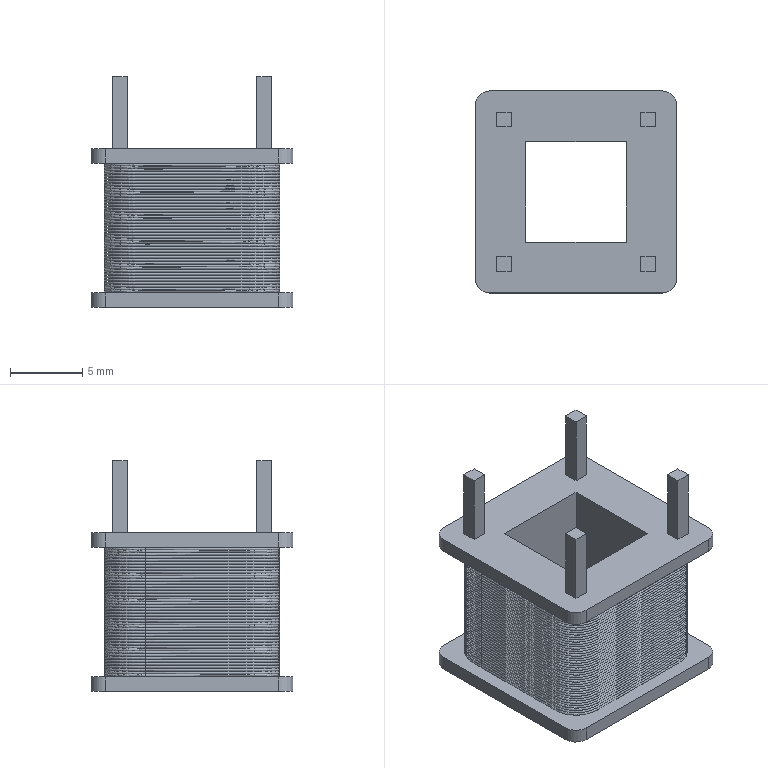Part | NX | features BREP 46 | 46 solids | 232 faces | box 14 x 14 x 16 mm | volume 814.621 mm3 | spline 180 | plane 40 | cylinder 12 | commonest cylinder face diameters 2 x12